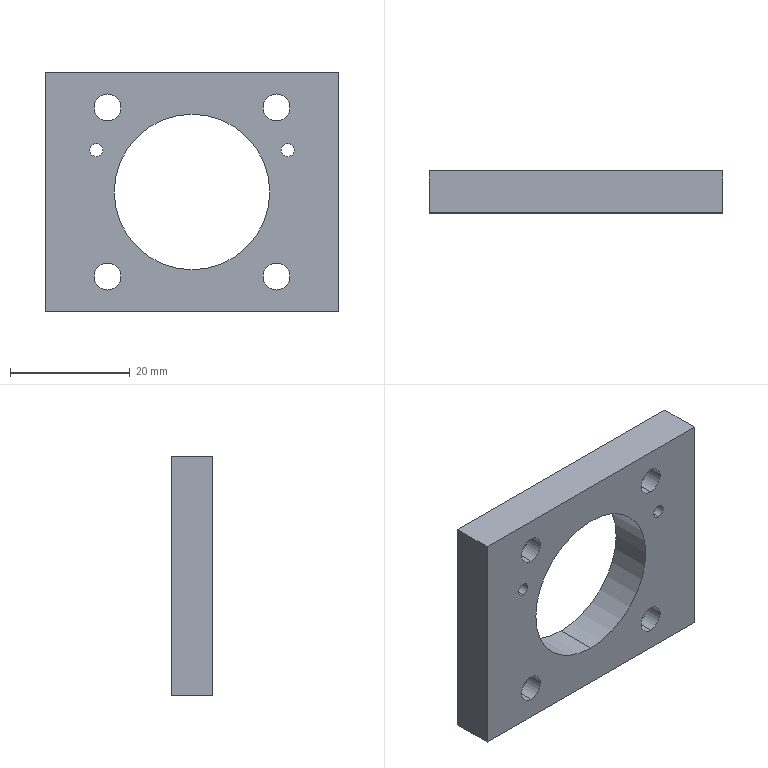Part | STEP file | SM140A-20-1140D-140A-600 Pressure plate | 1 solid | 32 faces | box 49 x 7 x 40 mm | volume 8955 mm3 | cylinder 22 | plane 10 | commonest cylinder face diameters 4.5 x8 8 x8 2.2 x4 26 x2